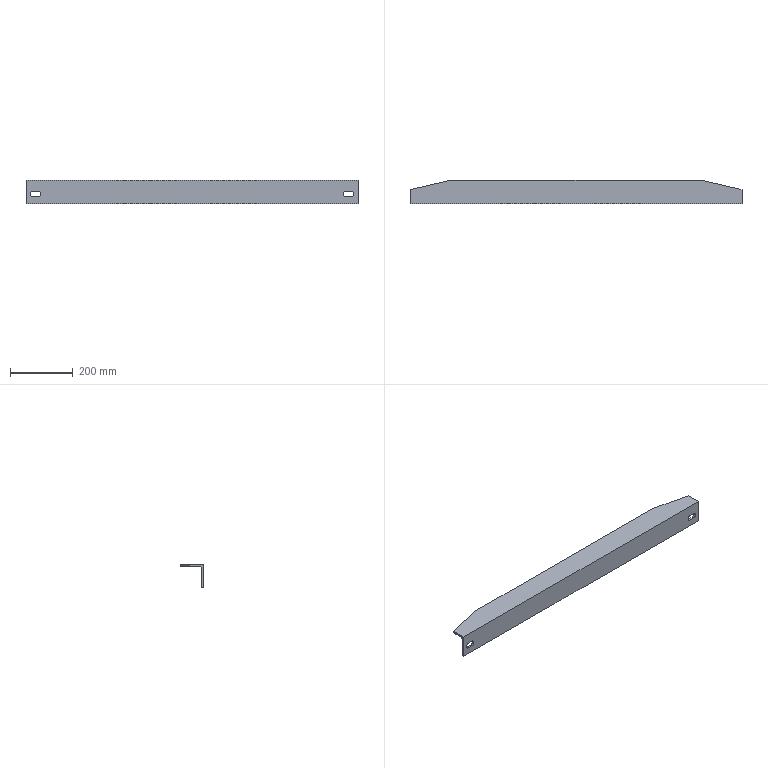Part | SolidWorks | features Chamfer 2, ICE 1, WeldMemberFeat 1, WeldmentFeature 1 | 1 solid | 21 faces | box 1056 x 75 x 75 mm | volume 899453 mm3 | plane 14 | cylinder 7 | commonest cylinder face diameters 18 x5 4 x2
STEP:
#1=CARTESIAN_POINT('',(398.,75.,-4.));
#2=VERTEX_POINT('',#1);
#3=CARTESIAN_POINT('',(-398.,75.,-4.));
#4=VERTEX_POINT('',#3);
#5=CARTESIAN_POINT('',(528.,75.,-4.));
#6=DIRECTION('',(-1.,0.,0.));
#7=VECTOR('',#6,1000.);
#8=LINE('',#5,#7);
#9=EDGE_CURVE('',#2,#4,#8,.T.);
#10=ORIENTED_EDGE('',*,*,#9,.T.);
#11=CARTESIAN_POINT('',(-398.,75.,0.));
#12=VERTEX_POINT('',#11);
#13=CARTESIAN_POINT('',(-398.,75.,0.));
#14=DIRECTION('',(0.,0.,1.));
#15=VECTOR('',#14,1000.);
#16=LINE('',#13,#15);
#17=EDGE_CURVE('',#4,#12,#16,.T.);
#18=ORIENTED_EDGE('',*,*,#17,.T.);
#19=CARTESIAN_POINT('',(398.,75.,0.));
#20=VERTEX_POINT('',#19);
#21=CARTESIAN_POINT('',(528.,75.,0.));
#22=DIRECTION('',(-1.,0.,0.));
#23=VECTOR('',#22,1000.);
#24=LINE('',#21,#23);
#25=EDGE_CURVE('',#20,#12,#24,.T.);
#26=ORIENTED_EDGE('',*,*,#25,.F.);
#27=CARTESIAN_POINT('',(398.,75.,0.));
#28=DIRECTION('',(0.,0.,-1.));
#29=VECTOR('',#28,1000.);
#30=LINE('',#27,#29);
#31=EDGE_CURVE('',#20,#2,#30,.T.);
#32=ORIENTED_EDGE('',*,*,#31,.T.);
#33=EDGE_LOOP('',(#10,#18,#26,#32));
#34=FACE_OUTER_BOUND('',#33,.T.);
#35=CARTESIAN_POINT('',(528.,75.,0.));
#36=DIRECTION('',(0.,-1.,0.));
#37=DIRECTION('',(0.,0.,-1.));
#38=AXIS2_PLACEMENT_3D('',#35,#36,#37);
#39=PLANE('',#38);
#40=ADVANCED_FACE('',(#34),#39,.F.);
#41=ORIENTED_EDGE('',*,*,#25,.T.);
#42=CARTESIAN_POINT('',(-528.,45.,0.));
#43=VERTEX_POINT('',#42);
#44=CARTESIAN_POINT('',(-398.,75.,0.));
#45=DIRECTION('',(-0.9744,-0.2249,0.));
#46=VECTOR('',#45,1000.);
#47=LINE('',#44,#46);
#48=EDGE_CURVE('',#12,#43,#47,.T.);
#49=ORIENTED_EDGE('',*,*,#48,.T.);
#50=CARTESIAN_POINT('',(-528.,0.,0.));
#51=VERTEX_POINT('',#50);
#52=CARTESIAN_POINT('',(-528.,75.,0.));
#53=DIRECTION('',(0.,-1.,0.));
#54=VECTOR('',#53,1000.);
#55=LINE('',#52,#54);
#56=EDGE_CURVE('',#43,#51,#55,.T.);
#57=ORIENTED_EDGE('',*,*,#56,.T.);
#58=CARTESIAN_POINT('',(528.,0.,0.));
#59=VERTEX_POINT('',#58);
#60=CARTESIAN_POINT('',(528.,0.,0.));
#61=DIRECTION('',(-1.,0.,0.));
#62=VECTOR('',#61,1000.);
#63=LINE('',#60,#62);
#64=EDGE_CURVE('',#59,#51,#63,.T.);
#65=ORIENTED_EDGE('',*,*,#64,.F.);
#66=CARTESIAN_POINT('',(528.,45.,0.));
#67=VERTEX_POINT('',#66);
#68=CARTESIAN_POINT('',(528.,75.,0.));
#69=DIRECTION('',(0.,-1.,0.));
#70=VECTOR('',#69,1000.);
#71=LINE('',#68,#70);
#72=EDGE_CURVE('',#67,#59,#71,.T.);
#73=ORIENTED_EDGE('',*,*,#72,.F.);
#74=CARTESIAN_POINT('',(528.,45.,0.));
#75=DIRECTION('',(-0.9744,0.2249,0.));
#76=VECTOR('',#75,1000.);
#77=LINE('',#74,#76);
#78=EDGE_CURVE('',#67,#20,#77,.T.);
#79=ORIENTED_EDGE('',*,*,#78,.T.);
#80=EDGE_LOOP('',(#41,#49,#57,#65,#73,#79));
#81=FACE_OUTER_BOUND('',#80,.T.);
#82=CARTESIAN_POINT('',(528.,75.,0.));
#83=DIRECTION('',(0.,0.,-1.));
#84=DIRECTION('',(0.,1.,0.));
#85=AXIS2_PLACEMENT_3D('',#82,#83,#84);
#86=PLANE('',#85);
#87=ADVANCED_FACE('',(#81),#86,.F.);
#88=CARTESIAN_POINT('',(-505.5,0.,-53.));
#89=VERTEX_POINT('',#88);
#90=CARTESIAN_POINT('',(-490.5,0.,-53.));
#91=VERTEX_POINT('',#90);
#92=CARTESIAN_POINT('',(-505.5,0.,-53.));
#93=DIRECTION('',(1.,0.,0.));
#94=VECTOR('',#93,1000.);
#95=LINE('',#92,#94);
#96=EDGE_CURVE('',#89,#91,#95,.T.);
#97=ORIENTED_EDGE('',*,*,#96,.F.);
#98=CARTESIAN_POINT('',(-505.5,0.,-35.));
#99=VERTEX_POINT('',#98);
#100=CARTESIAN_POINT('',(-505.5,0.,-44.));
#101=DIRECTION('',(0.,-1.,0.));
#102=DIRECTION('',(0.,0.,1.));
#103=AXIS2_PLACEMENT_3D('',#100,#101,#102);
#104=CIRCLE('',#103,9.);
#105=EDGE_CURVE('',#99,#89,#104,.T.);
#106=ORIENTED_EDGE('',*,*,#105,.F.);
#107=CARTESIAN_POINT('',(-490.5,0.,-35.));
#108=VERTEX_POINT('',#107);
#109=CARTESIAN_POINT('',(-505.5,0.,-35.));
#110=DIRECTION('',(-1.,0.,0.));
#111=VECTOR('',#110,1000.);
#112=LINE('',#109,#111);
#113=EDGE_CURVE('',#108,#99,#112,.T.);
#114=ORIENTED_EDGE('',*,*,#113,.F.);
#115=CARTESIAN_POINT('',(-490.5,0.,-44.));
#116=DIRECTION('',(0.,-1.,0.));
#117=DIRECTION('',(0.,0.,1.));
#118=AXIS2_PLACEMENT_3D('',#115,#116,#117);
#119=CIRCLE('',#118,9.);
#120=EDGE_CURVE('',#91,#108,#119,.T.);
#121=ORIENTED_EDGE('',*,*,#120,.F.);
#122=EDGE_LOOP('',(#97,#106,#114,#121));
#123=FACE_BOUND('',#122,.T.);
#124=CARTESIAN_POINT('',(490.5,0.,-53.));
#125=VERTEX_POINT('',#124);
#126=CARTESIAN_POINT('',(505.5,0.,-53.));
#127=VERTEX_POINT('',#126);
#128=CARTESIAN_POINT('',(490.5,0.,-53.));
#129=DIRECTION('',(1.,0.,0.));
#130=VECTOR('',#129,1000.);
#131=LINE('',#128,#130);
#132=EDGE_CURVE('',#125,#127,#131,.T.);
#133=ORIENTED_EDGE('',*,*,#132,.F.);
#134=CARTESIAN_POINT('',(490.5,0.,-35.));
#135=VERTEX_POINT('',#134);
#136=CARTESIAN_POINT('',(490.5,0.,-44.));
#137=DIRECTION('',(0.,-1.,0.));
#138=DIRECTION('',(0.,0.,1.));
#139=AXIS2_PLACEMENT_3D('',#136,#137,#138);
#140=CIRCLE('',#139,9.);
#141=EDGE_CURVE('',#135,#125,#140,.T.);
#142=ORIENTED_EDGE('',*,*,#141,.F.);
#143=CARTESIAN_POINT('',(505.5,0.,-35.));
#144=VERTEX_POINT('',#143);
#145=CARTESIAN_POINT('',(490.5,0.,-35.));
#146=DIRECTION('',(-1.,0.,0.));
#147=VECTOR('',#146,1000.);
#148=LINE('',#145,#147);
#149=EDGE_CURVE('',#144,#135,#148,.T.);
#150=ORIENTED_EDGE('',*,*,#149,.F.);
#151=CARTESIAN_POINT('',(505.5,0.,-44.));
#152=DIRECTION('',(0.,-1.,0.));
#153=DIRECTION('',(0.,0.,1.));
#154=AXIS2_PLACEMENT_3D('',#151,#152,#153);
#155=CIRCLE('',#154,9.);
#156=EDGE_CURVE('',#127,#144,#155,.T.);
#157=ORIENTED_EDGE('',*,*,#156,.F.);
#158=EDGE_LOOP('',(#133,#142,#150,#157));
#159=FACE_BOUND('',#158,.T.);
#160=CARTESIAN_POINT('',(-528.,0.,-75.));
#161=VERTEX_POINT('',#160);
#162=CARTESIAN_POINT('',(-528.,0.,0.));
#163=DIRECTION('',(0.,0.,-1.));
#164=VECTOR('',#163,1000.);
#165=LINE('',#162,#164);
#166=EDGE_CURVE('',#51,#161,#165,.T.);
#167=ORIENTED_EDGE('',*,*,#166,.T.);
#168=CARTESIAN_POINT('',(528.,0.,-75.));
#169=VERTEX_POINT('',#168);
#170=CARTESIAN_POINT('',(528.,0.,-75.));
#171=DIRECTION('',(-1.,0.,0.));
#172=VECTOR('',#171,1000.);
#173=LINE('',#170,#172);
#174=EDGE_CURVE('',#169,#161,#173,.T.);
#175=ORIENTED_EDGE('',*,*,#174,.F.);
#176=CARTESIAN_POINT('',(528.,0.,0.));
#177=DIRECTION('',(0.,0.,-1.));
#178=VECTOR('',#177,1000.);
#179=LINE('',#176,#178);
#180=EDGE_CURVE('',#59,#169,#179,.T.);
#181=ORIENTED_EDGE('',*,*,#180,.F.);
#182=ORIENTED_EDGE('',*,*,#64,.T.);
#183=EDGE_LOOP('',(#167,#175,#181,#182));
#184=FACE_OUTER_BOUND('',#183,.T.);
#185=CARTESIAN_POINT('',(528.,0.,0.));
#186=DIRECTION('',(0.,1.,0.));
#187=DIRECTION('',(0.,0.,1.));
#188=AXIS2_PLACEMENT_3D('',#185,#186,#187);
#189=PLANE('',#188);
#190=ADVANCED_FACE('',(#123,#159,#184),#189,.F.);
#191=CARTESIAN_POINT('',(-528.,4.,-75.));
#192=VERTEX_POINT('',#191);
#193=CARTESIAN_POINT('',(-528.,0.,-75.));
#194=DIRECTION('',(0.,1.,0.));
#195=VECTOR('',#194,1000.);
#196=LINE('',#193,#195);
#197=EDGE_CURVE('',#161,#192,#196,.T.);
#198=ORIENTED_EDGE('',*,*,#197,.T.);
#199=CARTESIAN_POINT('',(528.,4.,-75.));
#200=VERTEX_POINT('',#199);
#201=CARTESIAN_POINT('',(528.,4.,-75.));
#202=DIRECTION('',(-1.,0.,0.));
#203=VECTOR('',#202,1000.);
#204=LINE('',#201,#203);
#205=EDGE_CURVE('',#200,#192,#204,.T.);
#206=ORIENTED_EDGE('',*,*,#205,.F.);
#207=CARTESIAN_POINT('',(528.,0.,-75.));
#208=DIRECTION('',(0.,1.,0.));
#209=VECTOR('',#208,1000.);
#210=LINE('',#207,#209);
#211=EDGE_CURVE('',#169,#200,#210,.T.);
#212=ORIENTED_EDGE('',*,*,#211,.F.);
#213=ORIENTED_EDGE('',*,*,#174,.T.);
#214=EDGE_LOOP('',(#198,#206,#212,#213));
#215=FACE_OUTER_BOUND('',#214,.T.);
#216=CARTESIAN_POINT('',(528.,0.,-75.));
#217=DIRECTION('',(0.,0.,1.));
#218=DIRECTION('',(0.,-1.,0.));
#219=AXIS2_PLACEMENT_3D('',#216,#217,#218);
#220=PLANE('',#219);
#221=ADVANCED_FACE('',(#215),#220,.F.);
#222=CARTESIAN_POINT('',(-528.,6.,-73.));
#223=VERTEX_POINT('',#222);
#224=CARTESIAN_POINT('',(-528.,4.,-73.));
#225=DIRECTION('',(1.,0.,0.));
#226=DIRECTION('',(0.,0.,-1.));
#227=AXIS2_PLACEMENT_3D('',#224,#225,#226);
#228=CIRCLE('',#227,2.);
#229=EDGE_CURVE('',#192,#223,#228,.T.);
#230=ORIENTED_EDGE('',*,*,#229,.T.);
#231=CARTESIAN_POINT('',(528.,6.,-73.));
#232=VERTEX_POINT('',#231);
#233=CARTESIAN_POINT('',(528.,6.,-73.));
#234=DIRECTION('',(-1.,0.,0.));
#235=VECTOR('',#234,1000.);
#236=LINE('',#233,#235);
#237=EDGE_CURVE('',#232,#223,#236,.T.);
#238=ORIENTED_EDGE('',*,*,#237,.F.);
#239=CARTESIAN_POINT('',(528.,4.,-73.));
#240=DIRECTION('',(1.,0.,0.));
#241=DIRECTION('',(0.,0.,-1.));
#242=AXIS2_PLACEMENT_3D('',#239,#240,#241);
#243=CIRCLE('',#242,2.);
#244=EDGE_CURVE('',#200,#232,#243,.T.);
#245=ORIENTED_EDGE('',*,*,#244,.F.);
#246=ORIENTED_EDGE('',*,*,#205,.T.);
#247=EDGE_LOOP('',(#230,#238,#245,#246));
#248=FACE_OUTER_BOUND('',#247,.T.);
#249=CARTESIAN_POINT('',(528.,4.,-73.));
#250=DIRECTION('',(-1.,0.,0.));
#251=DIRECTION('',(0.,0.,1.));
#252=AXIS2_PLACEMENT_3D('',#249,#250,#251);
#253=CYLINDRICAL_SURFACE('',#252,2.);
#254=ADVANCED_FACE('',(#248),#253,.T.);
#255=CARTESIAN_POINT('',(-505.5,6.,-35.));
#256=VERTEX_POINT('',#255);
#257=CARTESIAN_POINT('',(-490.5,6.,-35.));
#258=VERTEX_POINT('',#257);
#259=CARTESIAN_POINT('',(-505.5,6.,-35.));
#260=DIRECTION('',(1.,0.,0.));
#261=VECTOR('',#260,1000.);
#262=LINE('',#259,#261);
#263=EDGE_CURVE('',#256,#258,#262,.T.);
#264=ORIENTED_EDGE('',*,*,#263,.F.);
#265=CARTESIAN_POINT('',(-505.5,6.,-53.));
#266=VERTEX_POINT('',#265);
#267=CARTESIAN_POINT('',(-505.5,6.,-44.));
#268=DIRECTION('',(0.,1.,0.));
#269=DIRECTION('',(0.,0.,1.));
#270=AXIS2_PLACEMENT_3D('',#267,#268,#269);
#271=CIRCLE('',#270,9.);
#272=EDGE_CURVE('',#266,#256,#271,.T.);
#273=ORIENTED_EDGE('',*,*,#272,.F.);
#274=CARTESIAN_POINT('',(-490.5,6.,-53.));
#275=VERTEX_POINT('',#274);
#276=CARTESIAN_POINT('',(-505.5,6.,-53.));
#277=DIRECTION('',(-1.,0.,0.));
#278=VECTOR('',#277,1000.);
#279=LINE('',#276,#278);
#280=EDGE_CURVE('',#275,#266,#279,.T.);
#281=ORIENTED_EDGE('',*,*,#280,.F.);
#282=CARTESIAN_POINT('',(-490.5,6.,-44.));
#283=DIRECTION('',(0.,1.,0.));
#284=DIRECTION('',(0.,0.,1.));
#285=AXIS2_PLACEMENT_3D('',#282,#283,#284);
#286=CIRCLE('',#285,9.);
#287=EDGE_CURVE('',#258,#275,#286,.T.);
#288=ORIENTED_EDGE('',*,*,#287,.F.);
#289=EDGE_LOOP('',(#264,#273,#281,#288));
#290=FACE_BOUND('',#289,.T.);
#291=CARTESIAN_POINT('',(490.5,6.,-35.));
#292=VERTEX_POINT('',#291);
#293=CARTESIAN_POINT('',(505.5,6.,-35.));
#294=VERTEX_POINT('',#293);
#295=CARTESIAN_POINT('',(490.5,6.,-35.));
#296=DIRECTION('',(1.,0.,0.));
#297=VECTOR('',#296,1000.);
#298=LINE('',#295,#297);
#299=EDGE_CURVE('',#292,#294,#298,.T.);
#300=ORIENTED_EDGE('',*,*,#299,.F.);
#301=CARTESIAN_POINT('',(490.5,6.,-53.));
#302=VERTEX_POINT('',#301);
#303=CARTESIAN_POINT('',(490.5,6.,-44.));
#304=DIRECTION('',(0.,1.,0.));
#305=DIRECTION('',(0.,0.,1.));
#306=AXIS2_PLACEMENT_3D('',#303,#304,#305);
#307=CIRCLE('',#306,9.);
#308=EDGE_CURVE('',#302,#292,#307,.T.);
#309=ORIENTED_EDGE('',*,*,#308,.F.);
#310=CARTESIAN_POINT('',(505.5,6.,-53.));
#311=VERTEX_POINT('',#310);
#312=CARTESIAN_POINT('',(490.5,6.,-53.));
#313=DIRECTION('',(-1.,0.,0.));
#314=VECTOR('',#313,1000.);
#315=LINE('',#312,#314);
#316=EDGE_CURVE('',#311,#302,#315,.T.);
#317=ORIENTED_EDGE('',*,*,#316,.F.);
#318=CARTESIAN_POINT('',(505.5,6.,-44.));
#319=DIRECTION('',(0.,1.,0.));
#320=DIRECTION('',(0.,0.,1.));
#321=AXIS2_PLACEMENT_3D('',#318,#319,#320);
#322=CIRCLE('',#321,9.);
#323=EDGE_CURVE('',#294,#311,#322,.T.);
#324=ORIENTED_EDGE('',*,*,#323,.F.);
#325=EDGE_LOOP('',(#300,#309,#317,#324));
#326=FACE_BOUND('',#325,.T.);
#327=CARTESIAN_POINT('',(-528.,6.,-15.));
#328=VERTEX_POINT('',#327);
#329=CARTESIAN_POINT('',(-528.,6.,-15.));
#330=DIRECTION('',(0.,0.,1.));
#331=VECTOR('',#330,1000.);
#332=LINE('',#329,#331);
#333=EDGE_CURVE('',#223,#328,#332,.T.);
#334=ORIENTED_EDGE('',*,*,#333,.T.);
#335=CARTESIAN_POINT('',(528.,6.,-15.));
#336=VERTEX_POINT('',#335);
#337=CARTESIAN_POINT('',(528.,6.,-15.));
#338=DIRECTION('',(-1.,0.,0.));
#339=VECTOR('',#338,1000.);
#340=LINE('',#337,#339);
#341=EDGE_CURVE('',#336,#328,#340,.T.);
#342=ORIENTED_EDGE('',*,*,#341,.F.);
#343=CARTESIAN_POINT('',(528.,6.,-15.));
#344=DIRECTION('',(0.,0.,1.));
#345=VECTOR('',#344,1000.);
#346=LINE('',#343,#345);
#347=EDGE_CURVE('',#232,#336,#346,.T.);
#348=ORIENTED_EDGE('',*,*,#347,.F.);
#349=ORIENTED_EDGE('',*,*,#237,.T.);
#350=EDGE_LOOP('',(#334,#342,#348,#349));
#351=FACE_OUTER_BOUND('',#350,.T.);
#352=CARTESIAN_POINT('',(528.,6.,-15.));
#353=DIRECTION('',(0.,-1.,0.));
#354=DIRECTION('',(0.,0.,-1.));
#355=AXIS2_PLACEMENT_3D('',#352,#353,#354);
#356=PLANE('',#355);
#357=ADVANCED_FACE('',(#290,#326,#351),#356,.F.);
#358=CARTESIAN_POINT('',(-528.,15.,-6.));
#359=VERTEX_POINT('',#358);
#360=CARTESIAN_POINT('',(-528.,15.,-15.));
#361=DIRECTION('',(-1.,0.,0.));
#362=DIRECTION('',(0.,0.,-1.));
#363=AXIS2_PLACEMENT_3D('',#360,#361,#362);
#364=CIRCLE('',#363,9.);
#365=EDGE_CURVE('',#328,#359,#364,.T.);
#366=ORIENTED_EDGE('',*,*,#365,.T.);
#367=CARTESIAN_POINT('',(528.,15.,-6.));
#368=VERTEX_POINT('',#367);
#369=CARTESIAN_POINT('',(528.,15.,-6.));
#370=DIRECTION('',(-1.,0.,0.));
#371=VECTOR('',#370,1000.);
#372=LINE('',#369,#371);
#373=EDGE_CURVE('',#368,#359,#372,.T.);
#374=ORIENTED_EDGE('',*,*,#373,.F.);
#375=CARTESIAN_POINT('',(528.,15.,-15.));
#376=DIRECTION('',(-1.,0.,0.));
#377=DIRECTION('',(0.,0.,-1.));
#378=AXIS2_PLACEMENT_3D('',#375,#376,#377);
#379=CIRCLE('',#378,9.);
#380=EDGE_CURVE('',#336,#368,#379,.T.);
#381=ORIENTED_EDGE('',*,*,#380,.F.);
#382=ORIENTED_EDGE('',*,*,#341,.T.);
#383=EDGE_LOOP('',(#366,#374,#381,#382));
#384=FACE_OUTER_BOUND('',#383,.T.);
#385=CARTESIAN_POINT('',(528.,15.,-15.));
#386=DIRECTION('',(-1.,0.,0.));
#387=DIRECTION('',(0.,0.,1.));
#388=AXIS2_PLACEMENT_3D('',#385,#386,#387);
#389=CYLINDRICAL_SURFACE('',#388,9.);
#390=ADVANCED_FACE('',(#384),#389,.F.);
#391=CARTESIAN_POINT('',(-528.,45.,-6.));
#392=VERTEX_POINT('',#391);
#393=CARTESIAN_POINT('',(-528.,73.,-6.));
#394=DIRECTION('',(0.,1.,0.));
#395=VECTOR('',#394,1000.);
#396=LINE('',#393,#395);
#397=EDGE_CURVE('',#359,#392,#396,.T.);
#398=ORIENTED_EDGE('',*,*,#397,.T.);
#399=CARTESIAN_POINT('',(-406.667,73.,-6.));
#400=VERTEX_POINT('',#399);
#401=CARTESIAN_POINT('',(-398.,75.,-6.));
#402=DIRECTION('',(0.9744,0.2249,0.));
#403=VECTOR('',#402,1000.);
#404=LINE('',#401,#403);
#405=EDGE_CURVE('',#392,#400,#404,.T.);
#406=ORIENTED_EDGE('',*,*,#405,.T.);
#407=CARTESIAN_POINT('',(406.667,73.,-6.));
#408=VERTEX_POINT('',#407);
#409=CARTESIAN_POINT('',(528.,73.,-6.));
#410=DIRECTION('',(-1.,0.,0.));
#411=VECTOR('',#410,1000.);
#412=LINE('',#409,#411);
#413=EDGE_CURVE('',#408,#400,#412,.T.);
#414=ORIENTED_EDGE('',*,*,#413,.F.);
#415=CARTESIAN_POINT('',(528.,45.,-6.));
#416=VERTEX_POINT('',#415);
#417=CARTESIAN_POINT('',(528.,45.,-6.));
#418=DIRECTION('',(0.9744,-0.2249,0.));
#419=VECTOR('',#418,1000.);
#420=LINE('',#417,#419);
#421=EDGE_CURVE('',#408,#416,#420,.T.);
#422=ORIENTED_EDGE('',*,*,#421,.T.);
#423=CARTESIAN_POINT('',(528.,73.,-6.));
#424=DIRECTION('',(0.,1.,0.));
#425=VECTOR('',#424,1000.);
#426=LINE('',#423,#425);
#427=EDGE_CURVE('',#368,#416,#426,.T.);
#428=ORIENTED_EDGE('',*,*,#427,.F.);
#429=ORIENTED_EDGE('',*,*,#373,.T.);
#430=EDGE_LOOP('',(#398,#406,#414,#422,#428,#429));
#431=FACE_OUTER_BOUND('',#430,.T.);
#432=CARTESIAN_POINT('',(528.,73.,-6.));
#433=DIRECTION('',(0.,0.,1.));
#434=DIRECTION('',(0.,-1.,0.));
#435=AXIS2_PLACEMENT_3D('',#432,#433,#434);
#436=PLANE('',#435);
#437=ADVANCED_FACE('',(#431),#436,.F.);
#438=ORIENTED_EDGE('',*,*,#413,.T.);
#439=CARTESIAN_POINT('',(-406.667,73.,-6.));
#440=CARTESIAN_POINT('',(-401.59,74.172,-6.));
#441=CARTESIAN_POINT('',(-398.,75.,-5.172));
#442=CARTESIAN_POINT('',(-398.,75.,-4.));
#443=(BOUNDED_CURVE()B_SPLINE_CURVE(3,(#439,#440,#441,#442),.UNSPECIFIED.,.F.,.F.)B_SPLINE_CURVE_WITH_KNOTS((4,4),(1.571,3.142),.UNSPECIFIED.)CURVE()GEOMETRIC_REPRESENTATION_ITEM()RATIONAL_B_SPLINE_CURVE((1.,0.8047,0.8047,1.))REPRESENTATION_ITEM(''));
#444=EDGE_CURVE('',#400,#4,#443,.T.);
#445=ORIENTED_EDGE('',*,*,#444,.T.);
#446=ORIENTED_EDGE('',*,*,#9,.F.);
#447=CARTESIAN_POINT('',(398.,75.,-4.));
#448=CARTESIAN_POINT('',(398.,75.,-5.172));
#449=CARTESIAN_POINT('',(401.59,74.172,-6.));
#450=CARTESIAN_POINT('',(406.667,73.,-6.));
#451=(BOUNDED_CURVE()B_SPLINE_CURVE(3,(#447,#448,#449,#450),.UNSPECIFIED.,.F.,.F.)B_SPLINE_CURVE_WITH_KNOTS((4,4),(0.,1.571),.UNSPECIFIED.)CURVE()GEOMETRIC_REPRESENTATION_ITEM()RATIONAL_B_SPLINE_CURVE((1.,0.8047,0.8047,1.))REPRESENTATION_ITEM(''));
#452=EDGE_CURVE('',#2,#408,#451,.T.);
#453=ORIENTED_EDGE('',*,*,#452,.T.);
#454=EDGE_LOOP('',(#438,#445,#446,#453));
#455=FACE_OUTER_BOUND('',#454,.T.);
#456=CARTESIAN_POINT('',(528.,73.,-4.));
#457=DIRECTION('',(-1.,0.,0.));
#458=DIRECTION('',(0.,0.,1.));
#459=AXIS2_PLACEMENT_3D('',#456,#457,#458);
#460=CYLINDRICAL_SURFACE('',#459,2.);
#461=ADVANCED_FACE('',(#455),#460,.T.);
#462=ORIENTED_EDGE('',*,*,#427,.T.);
#463=CARTESIAN_POINT('',(528.,45.,-4.));
#464=DIRECTION('',(0.,0.,1.));
#465=VECTOR('',#464,1000.);
#466=LINE('',#463,#465);
#467=EDGE_CURVE('',#416,#67,#466,.T.);
#468=ORIENTED_EDGE('',*,*,#467,.T.);
#469=ORIENTED_EDGE('',*,*,#72,.T.);
#470=ORIENTED_EDGE('',*,*,#180,.T.);
#471=ORIENTED_EDGE('',*,*,#211,.T.);
#472=ORIENTED_EDGE('',*,*,#244,.T.);
#473=ORIENTED_EDGE('',*,*,#347,.T.);
#474=ORIENTED_EDGE('',*,*,#380,.T.);
#475=EDGE_LOOP('',(#462,#468,#469,#470,#471,#472,#473,#474));
#476=FACE_OUTER_BOUND('',#475,.T.);
#477=CARTESIAN_POINT('',(528.,73.,-4.));
#478=DIRECTION('',(-1.,0.,0.));
#479=DIRECTION('',(0.,0.,1.));
#480=AXIS2_PLACEMENT_3D('',#477,#478,#479);
#481=PLANE('',#480);
#482=ADVANCED_FACE('',(#476),#481,.F.);
#483=ORIENTED_EDGE('',*,*,#56,.F.);
#484=CARTESIAN_POINT('',(-528.,45.,-4.));
#485=DIRECTION('',(0.,0.,-1.));
#486=VECTOR('',#485,1000.);
#487=LINE('',#484,#486);
#488=EDGE_CURVE('',#43,#392,#487,.T.);
#489=ORIENTED_EDGE('',*,*,#488,.T.);
#490=ORIENTED_EDGE('',*,*,#397,.F.);
#491=ORIENTED_EDGE('',*,*,#365,.F.);
#492=ORIENTED_EDGE('',*,*,#333,.F.);
#493=ORIENTED_EDGE('',*,*,#229,.F.);
#494=ORIENTED_EDGE('',*,*,#197,.F.);
#495=ORIENTED_EDGE('',*,*,#166,.F.);
#496=EDGE_LOOP('',(#483,#489,#490,#491,#492,#493,#494,#495));
#497=FACE_OUTER_BOUND('',#496,.T.);
#498=CARTESIAN_POINT('',(-528.,73.,-4.));
#499=DIRECTION('',(-1.,0.,0.));
#500=DIRECTION('',(0.,0.,1.));
#501=AXIS2_PLACEMENT_3D('',#498,#499,#500);
#502=PLANE('',#501);
#503=ADVANCED_FACE('',(#497),#502,.T.);
#504=ORIENTED_EDGE('',*,*,#141,.T.);
#505=CARTESIAN_POINT('',(490.5,-0.001,-53.));
#506=DIRECTION('',(0.,1.,0.));
#507=VECTOR('',#506,1000.);
#508=LINE('',#505,#507);
#509=EDGE_CURVE('',#125,#302,#508,.T.);
#510=ORIENTED_EDGE('',*,*,#509,.T.);
#511=ORIENTED_EDGE('',*,*,#308,.T.);
#512=CARTESIAN_POINT('',(490.5,-0.001,-35.));
#513=DIRECTION('',(0.,1.,0.));
#514=VECTOR('',#513,1000.);
#515=LINE('',#512,#514);
#516=EDGE_CURVE('',#135,#292,#515,.T.);
#517=ORIENTED_EDGE('',*,*,#516,.F.);
#518=EDGE_LOOP('',(#504,#510,#511,#517));
#519=FACE_OUTER_BOUND('',#518,.T.);
#520=CARTESIAN_POINT('',(490.5,-0.001,-44.));
#521=DIRECTION('',(0.,1.,0.));
#522=DIRECTION('',(0.,0.,1.));
#523=AXIS2_PLACEMENT_3D('',#520,#521,#522);
#524=CYLINDRICAL_SURFACE('',#523,9.);
#525=ADVANCED_FACE('',(#519),#524,.F.);
#526=ORIENTED_EDGE('',*,*,#132,.T.);
#527=CARTESIAN_POINT('',(505.5,-0.001,-53.));
#528=DIRECTION('',(0.,1.,0.));
#529=VECTOR('',#528,1000.);
#530=LINE('',#527,#529);
#531=EDGE_CURVE('',#127,#311,#530,.T.);
#532=ORIENTED_EDGE('',*,*,#531,.T.);
#533=ORIENTED_EDGE('',*,*,#316,.T.);
#534=ORIENTED_EDGE('',*,*,#509,.F.);
#535=EDGE_LOOP('',(#526,#532,#533,#534));
#536=FACE_OUTER_BOUND('',#535,.T.);
#537=CARTESIAN_POINT('',(490.5,-0.001,-53.));
#538=DIRECTION('',(0.,0.,-1.));
#539=DIRECTION('',(0.,1.,0.));
#540=AXIS2_PLACEMENT_3D('',#537,#538,#539);
#541=PLANE('',#540);
#542=ADVANCED_FACE('',(#536),#541,.F.);
#543=ORIENTED_EDGE('',*,*,#156,.T.);
#544=CARTESIAN_POINT('',(505.5,-0.001,-35.));
#545=DIRECTION('',(0.,1.,0.));
#546=VECTOR('',#545,1000.);
#547=LINE('',#544,#546);
#548=EDGE_CURVE('',#144,#294,#547,.T.);
#549=ORIENTED_EDGE('',*,*,#548,.T.);
#550=ORIENTED_EDGE('',*,*,#323,.T.);
#551=ORIENTED_EDGE('',*,*,#531,.F.);
#552=EDGE_LOOP('',(#543,#549,#550,#551));
#553=FACE_OUTER_BOUND('',#552,.T.);
#554=CARTESIAN_POINT('',(505.5,-0.001,-44.));
#555=DIRECTION('',(0.,1.,0.));
#556=DIRECTION('',(0.,0.,1.));
#557=AXIS2_PLACEMENT_3D('',#554,#555,#556);
#558=CYLINDRICAL_SURFACE('',#557,9.);
#559=ADVANCED_FACE('',(#553),#558,.F.);
#560=ORIENTED_EDGE('',*,*,#149,.T.);
#561=ORIENTED_EDGE('',*,*,#516,.T.);
#562=ORIENTED_EDGE('',*,*,#299,.T.);
#563=ORIENTED_EDGE('',*,*,#548,.F.);
#564=EDGE_LOOP('',(#560,#561,#562,#563));
#565=FACE_OUTER_BOUND('',#564,.T.);
#566=CARTESIAN_POINT('',(490.5,-0.001,-35.));
#567=DIRECTION('',(0.,0.,1.));
#568=DIRECTION('',(0.,-1.,0.));
#569=AXIS2_PLACEMENT_3D('',#566,#567,#568);
#570=PLANE('',#569);
#571=ADVANCED_FACE('',(#565),#570,.F.);
#572=ORIENTED_EDGE('',*,*,#105,.T.);
#573=CARTESIAN_POINT('',(-505.5,-0.001,-53.));
#574=DIRECTION('',(0.,1.,0.));
#575=VECTOR('',#574,1000.);
#576=LINE('',#573,#575);
#577=EDGE_CURVE('',#89,#266,#576,.T.);
#578=ORIENTED_EDGE('',*,*,#577,.T.);
#579=ORIENTED_EDGE('',*,*,#272,.T.);
#580=CARTESIAN_POINT('',(-505.5,-0.001,-35.));
#581=DIRECTION('',(0.,1.,0.));
#582=VECTOR('',#581,1000.);
#583=LINE('',#580,#582);
#584=EDGE_CURVE('',#99,#256,#583,.T.);
#585=ORIENTED_EDGE('',*,*,#584,.F.);
#586=EDGE_LOOP('',(#572,#578,#579,#585));
#587=FACE_OUTER_BOUND('',#586,.T.);
#588=CARTESIAN_POINT('',(-505.5,-0.001,-44.));
#589=DIRECTION('',(0.,1.,0.));
#590=DIRECTION('',(0.,0.,1.));
#591=AXIS2_PLACEMENT_3D('',#588,#589,#590);
#592=CYLINDRICAL_SURFACE('',#591,9.);
#593=ADVANCED_FACE('',(#587),#592,.F.);
#594=ORIENTED_EDGE('',*,*,#96,.T.);
#595=CARTESIAN_POINT('',(-490.5,-0.001,-53.));
#596=DIRECTION('',(0.,1.,0.));
#597=VECTOR('',#596,1000.);
#598=LINE('',#595,#597);
#599=EDGE_CURVE('',#91,#275,#598,.T.);
#600=ORIENTED_EDGE('',*,*,#599,.T.);
#601=ORIENTED_EDGE('',*,*,#280,.T.);
#602=ORIENTED_EDGE('',*,*,#577,.F.);
#603=EDGE_LOOP('',(#594,#600,#601,#602));
#604=FACE_OUTER_BOUND('',#603,.T.);
#605=CARTESIAN_POINT('',(-505.5,-0.001,-53.));
#606=DIRECTION('',(0.,0.,-1.));
#607=DIRECTION('',(-1.,0.,0.));
#608=AXIS2_PLACEMENT_3D('',#605,#606,#607);
#609=PLANE('',#608);
#610=ADVANCED_FACE('',(#604),#609,.F.);
#611=ORIENTED_EDGE('',*,*,#120,.T.);
#612=CARTESIAN_POINT('',(-490.5,-0.001,-35.));
#613=DIRECTION('',(0.,1.,0.));
#614=VECTOR('',#613,1000.);
#615=LINE('',#612,#614);
#616=EDGE_CURVE('',#108,#258,#615,.T.);
#617=ORIENTED_EDGE('',*,*,#616,.T.);
#618=ORIENTED_EDGE('',*,*,#287,.T.);
#619=ORIENTED_EDGE('',*,*,#599,.F.);
#620=EDGE_LOOP('',(#611,#617,#618,#619));
#621=FACE_OUTER_BOUND('',#620,.T.);
#622=CARTESIAN_POINT('',(-490.5,-0.001,-44.));
#623=DIRECTION('',(0.,1.,0.));
#624=DIRECTION('',(0.,0.,1.));
#625=AXIS2_PLACEMENT_3D('',#622,#623,#624);
#626=CYLINDRICAL_SURFACE('',#625,9.);
#627=ADVANCED_FACE('',(#621),#626,.F.);
#628=ORIENTED_EDGE('',*,*,#113,.T.);
#629=ORIENTED_EDGE('',*,*,#584,.T.);
#630=ORIENTED_EDGE('',*,*,#263,.T.);
#631=ORIENTED_EDGE('',*,*,#616,.F.);
#632=EDGE_LOOP('',(#628,#629,#630,#631));
#633=FACE_OUTER_BOUND('',#632,.T.);
#634=CARTESIAN_POINT('',(-505.5,-0.001,-35.));
#635=DIRECTION('',(0.,0.,1.));
#636=DIRECTION('',(0.,-1.,0.));
#637=AXIS2_PLACEMENT_3D('',#634,#635,#636);
#638=PLANE('',#637);
#639=ADVANCED_FACE('',(#633),#638,.F.);
#640=ORIENTED_EDGE('',*,*,#452,.F.);
#641=ORIENTED_EDGE('',*,*,#31,.F.);
#642=ORIENTED_EDGE('',*,*,#78,.F.);
#643=ORIENTED_EDGE('',*,*,#467,.F.);
#644=ORIENTED_EDGE('',*,*,#421,.F.);
#645=EDGE_LOOP('',(#640,#641,#642,#643,#644));
#646=FACE_OUTER_BOUND('',#645,.T.);
#647=CARTESIAN_POINT('',(528.,45.,-4.));
#648=DIRECTION('',(-0.2249,-0.9744,0.));
#649=DIRECTION('',(0.,0.,1.));
#650=AXIS2_PLACEMENT_3D('',#647,#648,#649);
#651=PLANE('',#650);
#652=ADVANCED_FACE('',(#646),#651,.F.);
#653=ORIENTED_EDGE('',*,*,#405,.F.);
#654=ORIENTED_EDGE('',*,*,#488,.F.);
#655=ORIENTED_EDGE('',*,*,#48,.F.);
#656=ORIENTED_EDGE('',*,*,#17,.F.);
#657=ORIENTED_EDGE('',*,*,#444,.F.);
#658=EDGE_LOOP('',(#653,#654,#655,#656,#657));
#659=FACE_OUTER_BOUND('',#658,.T.);
#660=CARTESIAN_POINT('',(-398.,75.,0.));
#661=DIRECTION('',(-0.2249,0.9744,0.));
#662=DIRECTION('',(0.,0.,-1.));
#663=AXIS2_PLACEMENT_3D('',#660,#661,#662);
#664=PLANE('',#663);
#665=ADVANCED_FACE('',(#659),#664,.T.);
#666=CLOSED_SHELL('',(#40,#87,#190,#221,#254,#357,#390,#437,#461,#482,#503,#525,#542,#559,#571,#593,#610,#627,#639,#652,#665));
#667=MANIFOLD_SOLID_BREP('',#666);
#668=CARTESIAN_POINT('',(0.,0.,0.));
#669=DIRECTION('',(0.,0.,1.));
#670=DIRECTION('',(1.,0.,0.));
#671=AXIS2_PLACEMENT_3D('',#668,#669,#670);
#672=(LENGTH_UNIT()NAMED_UNIT(*)SI_UNIT(.MILLI.,.METRE.));
#673=UNCERTAINTY_MEASURE_WITH_UNIT(LENGTH_MEASURE(0.00001),#672,'','');
#674=(NAMED_UNIT(*)PLANE_ANGLE_UNIT()SI_UNIT($,.RADIAN.));
#675=(NAMED_UNIT(*)SI_UNIT($,.STERADIAN.)SOLID_ANGLE_UNIT());
#676=(GEOMETRIC_REPRESENTATION_CONTEXT(3)GLOBAL_UNCERTAINTY_ASSIGNED_CONTEXT((#673))GLOBAL_UNIT_ASSIGNED_CONTEXT((#672,#674,#675))REPRESENTATION_CONTEXT('',''));
#677=ADVANCED_BREP_SHAPE_REPRESENTATION('',(#667,#671),#676);